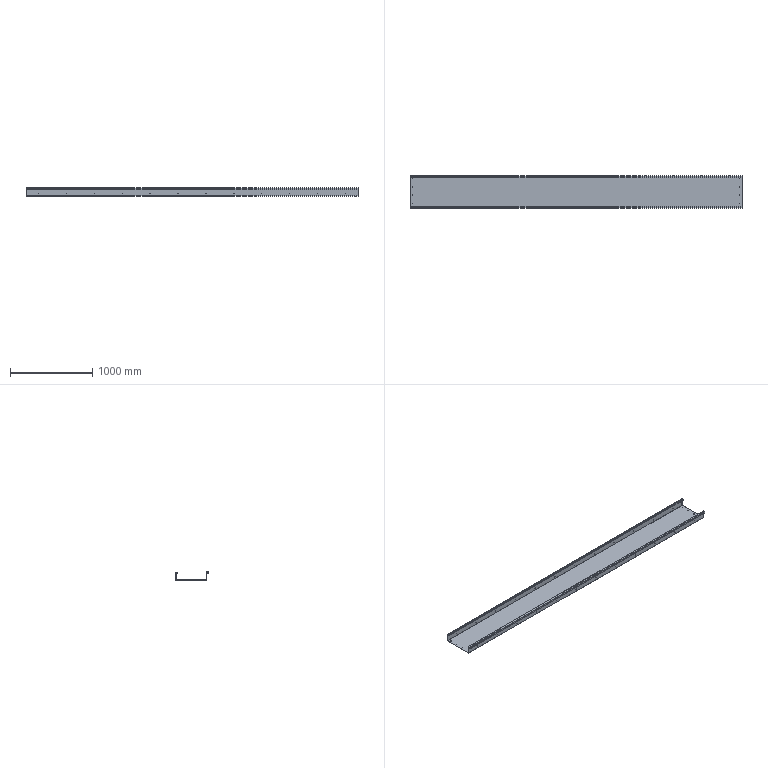Part | STEP file | TS-S81 | 1 solid | 118 faces | box 4045 x 393 x 100 mm | volume 5094556 mm3 | cylinder 76 | plane 42 | commonest cylinder face diameters 5.4 x48 5 x16 0.4 x6 4.4 x6